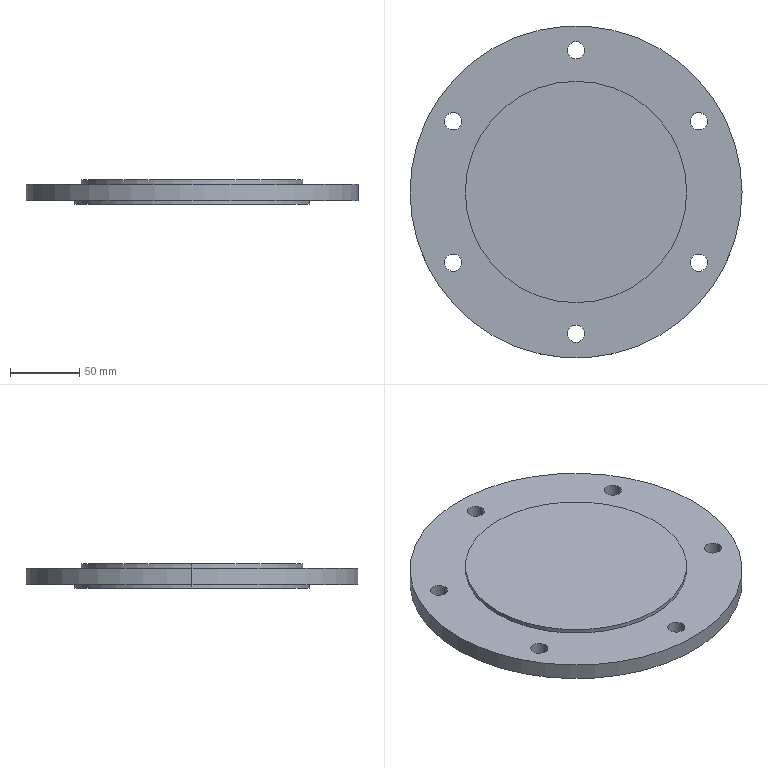Part | SolidWorks | features ICE 3, HoleWzd 2, Revolution 1 | 1 solid | 28 faces | box 240 x 240 x 17.5 mm | volume 563209 mm3 | cylinder 22 | plane 6 | commonest cylinder face diameters 12.5 x12 100 x2 130 x2 160 x2 170 x2 240 x2
STEP:
#1=CARTESIAN_POINT('',(586.231,234.744,-152.193));
#2=VERTEX_POINT('',#1);
#3=CARTESIAN_POINT('',(456.231,234.744,-152.193));
#4=VERTEX_POINT('',#3);
#5=CARTESIAN_POINT('',(521.231,234.744,-152.193));
#6=DIRECTION('',(0.,0.,-1.));
#7=DIRECTION('',(-1.,0.,0.));
#8=AXIS2_PLACEMENT_3D('',#5,#6,#7);
#9=CIRCLE('',#8,65.);
#10=EDGE_CURVE('',#2,#4,#9,.T.);
#11=ORIENTED_EDGE('',*,*,#10,.F.);
#12=CARTESIAN_POINT('',(586.231,234.744,-153.193));
#13=VERTEX_POINT('',#12);
#14=CARTESIAN_POINT('',(586.231,234.744,-153.193));
#15=DIRECTION('',(0.,0.,-1.));
#16=VECTOR('',#15,1000.);
#17=LINE('',#14,#16);
#18=EDGE_CURVE('',#2,#13,#17,.T.);
#19=ORIENTED_EDGE('',*,*,#18,.T.);
#20=CARTESIAN_POINT('',(456.231,234.744,-153.193));
#21=VERTEX_POINT('',#20);
#22=CARTESIAN_POINT('',(521.231,234.744,-153.193));
#23=DIRECTION('',(0.,0.,-1.));
#24=DIRECTION('',(-1.,0.,0.));
#25=AXIS2_PLACEMENT_3D('',#22,#23,#24);
#26=CIRCLE('',#25,65.);
#27=EDGE_CURVE('',#13,#21,#26,.T.);
#28=ORIENTED_EDGE('',*,*,#27,.T.);
#29=CARTESIAN_POINT('',(456.231,234.744,-153.193));
#30=DIRECTION('',(0.,0.,-1.));
#31=VECTOR('',#30,1000.);
#32=LINE('',#29,#31);
#33=EDGE_CURVE('',#4,#21,#32,.T.);
#34=ORIENTED_EDGE('',*,*,#33,.F.);
#35=EDGE_LOOP('',(#11,#19,#28,#34));
#36=FACE_OUTER_BOUND('',#35,.T.);
#37=CARTESIAN_POINT('',(521.231,234.744,-153.193));
#38=DIRECTION('',(0.,0.,-1.));
#39=DIRECTION('',(-1.,0.,0.));
#40=AXIS2_PLACEMENT_3D('',#37,#38,#39);
#41=CYLINDRICAL_SURFACE('',#40,65.);
#42=ADVANCED_FACE('',(#36),#41,.F.);
#43=CARTESIAN_POINT('',(527.481,337.244,-150.693));
#44=VERTEX_POINT('',#43);
#45=CARTESIAN_POINT('',(514.981,337.244,-150.693));
#46=VERTEX_POINT('',#45);
#47=CARTESIAN_POINT('',(521.231,337.244,-150.693));
#48=DIRECTION('',(0.,0.,-1.));
#49=DIRECTION('',(-1.,0.,0.));
#50=AXIS2_PLACEMENT_3D('',#47,#48,#49);
#51=CIRCLE('',#50,6.25);
#52=EDGE_CURVE('',#44,#46,#51,.T.);
#53=ORIENTED_EDGE('',*,*,#52,.T.);
#54=CARTESIAN_POINT('',(514.981,337.244,-138.693));
#55=VERTEX_POINT('',#54);
#56=CARTESIAN_POINT('',(514.981,337.244,-138.693));
#57=DIRECTION('',(0.,0.,1.));
#58=VECTOR('',#57,1000.);
#59=LINE('',#56,#58);
#60=EDGE_CURVE('',#46,#55,#59,.T.);
#61=ORIENTED_EDGE('',*,*,#60,.T.);
#62=CARTESIAN_POINT('',(527.481,337.244,-138.693));
#63=VERTEX_POINT('',#62);
#64=CARTESIAN_POINT('',(521.231,337.244,-138.693));
#65=DIRECTION('',(0.,0.,1.));
#66=DIRECTION('',(1.,0.,0.));
#67=AXIS2_PLACEMENT_3D('',#64,#65,#66);
#68=CIRCLE('',#67,6.25);
#69=EDGE_CURVE('',#55,#63,#68,.T.);
#70=ORIENTED_EDGE('',*,*,#69,.T.);
#71=CARTESIAN_POINT('',(527.481,337.244,-138.693));
#72=DIRECTION('',(0.,0.,1.));
#73=VECTOR('',#72,1000.);
#74=LINE('',#71,#73);
#75=EDGE_CURVE('',#44,#63,#74,.T.);
#76=ORIENTED_EDGE('',*,*,#75,.F.);
#77=EDGE_LOOP('',(#53,#61,#70,#76));
#78=FACE_OUTER_BOUND('',#77,.T.);
#79=CARTESIAN_POINT('',(521.231,337.244,-138.693));
#80=DIRECTION('',(0.,0.,1.));
#81=DIRECTION('',(1.,0.,0.));
#82=AXIS2_PLACEMENT_3D('',#79,#80,#81);
#83=CYLINDRICAL_SURFACE('',#82,6.25);
#84=ADVANCED_FACE('',(#78),#83,.F.);
#85=CARTESIAN_POINT('',(616.248,285.994,-150.693));
#86=VERTEX_POINT('',#85);
#87=CARTESIAN_POINT('',(603.748,285.994,-150.693));
#88=VERTEX_POINT('',#87);
#89=CARTESIAN_POINT('',(609.998,285.994,-150.693));
#90=DIRECTION('',(0.,0.,-1.));
#91=DIRECTION('',(-1.,0.,0.));
#92=AXIS2_PLACEMENT_3D('',#89,#90,#91);
#93=CIRCLE('',#92,6.25);
#94=EDGE_CURVE('',#86,#88,#93,.T.);
#95=ORIENTED_EDGE('',*,*,#94,.T.);
#96=CARTESIAN_POINT('',(603.748,285.994,-138.693));
#97=VERTEX_POINT('',#96);
#98=CARTESIAN_POINT('',(603.748,285.994,-138.693));
#99=DIRECTION('',(0.,0.,1.));
#100=VECTOR('',#99,1000.);
#101=LINE('',#98,#100);
#102=EDGE_CURVE('',#88,#97,#101,.T.);
#103=ORIENTED_EDGE('',*,*,#102,.T.);
#104=CARTESIAN_POINT('',(616.248,285.994,-138.693));
#105=VERTEX_POINT('',#104);
#106=CARTESIAN_POINT('',(609.998,285.994,-138.693));
#107=DIRECTION('',(0.,0.,1.));
#108=DIRECTION('',(1.,0.,0.));
#109=AXIS2_PLACEMENT_3D('',#106,#107,#108);
#110=CIRCLE('',#109,6.25);
#111=EDGE_CURVE('',#97,#105,#110,.T.);
#112=ORIENTED_EDGE('',*,*,#111,.T.);
#113=CARTESIAN_POINT('',(616.248,285.994,-138.693));
#114=DIRECTION('',(0.,0.,1.));
#115=VECTOR('',#114,1000.);
#116=LINE('',#113,#115);
#117=EDGE_CURVE('',#86,#105,#116,.T.);
#118=ORIENTED_EDGE('',*,*,#117,.F.);
#119=EDGE_LOOP('',(#95,#103,#112,#118));
#120=FACE_OUTER_BOUND('',#119,.T.);
#121=CARTESIAN_POINT('',(609.998,285.994,-138.693));
#122=DIRECTION('',(0.,0.,1.));
#123=DIRECTION('',(1.,0.,0.));
#124=AXIS2_PLACEMENT_3D('',#121,#122,#123);
#125=CYLINDRICAL_SURFACE('',#124,6.25);
#126=ADVANCED_FACE('',(#120),#125,.F.);
#127=CARTESIAN_POINT('',(438.713,285.994,-150.693));
#128=VERTEX_POINT('',#127);
#129=CARTESIAN_POINT('',(426.213,285.994,-150.693));
#130=VERTEX_POINT('',#129);
#131=CARTESIAN_POINT('',(432.463,285.994,-150.693));
#132=DIRECTION('',(0.,0.,-1.));
#133=DIRECTION('',(-1.,0.,0.));
#134=AXIS2_PLACEMENT_3D('',#131,#132,#133);
#135=CIRCLE('',#134,6.25);
#136=EDGE_CURVE('',#128,#130,#135,.T.);
#137=ORIENTED_EDGE('',*,*,#136,.T.);
#138=CARTESIAN_POINT('',(426.213,285.994,-138.693));
#139=VERTEX_POINT('',#138);
#140=CARTESIAN_POINT('',(426.213,285.994,-138.693));
#141=DIRECTION('',(0.,0.,1.));
#142=VECTOR('',#141,1000.);
#143=LINE('',#140,#142);
#144=EDGE_CURVE('',#130,#139,#143,.T.);
#145=ORIENTED_EDGE('',*,*,#144,.T.);
#146=CARTESIAN_POINT('',(438.713,285.994,-138.693));
#147=VERTEX_POINT('',#146);
#148=CARTESIAN_POINT('',(432.463,285.994,-138.693));
#149=DIRECTION('',(0.,0.,1.));
#150=DIRECTION('',(1.,0.,0.));
#151=AXIS2_PLACEMENT_3D('',#148,#149,#150);
#152=CIRCLE('',#151,6.25);
#153=EDGE_CURVE('',#139,#147,#152,.T.);
#154=ORIENTED_EDGE('',*,*,#153,.T.);
#155=CARTESIAN_POINT('',(438.713,285.994,-138.693));
#156=DIRECTION('',(0.,0.,1.));
#157=VECTOR('',#156,1000.);
#158=LINE('',#155,#157);
#159=EDGE_CURVE('',#128,#147,#158,.T.);
#160=ORIENTED_EDGE('',*,*,#159,.F.);
#161=EDGE_LOOP('',(#137,#145,#154,#160));
#162=FACE_OUTER_BOUND('',#161,.T.);
#163=CARTESIAN_POINT('',(432.463,285.994,-138.693));
#164=DIRECTION('',(0.,0.,1.));
#165=DIRECTION('',(1.,0.,0.));
#166=AXIS2_PLACEMENT_3D('',#163,#164,#165);
#167=CYLINDRICAL_SURFACE('',#166,6.25);
#168=ADVANCED_FACE('',(#162),#167,.F.);
#169=CARTESIAN_POINT('',(438.713,183.494,-150.693));
#170=VERTEX_POINT('',#169);
#171=CARTESIAN_POINT('',(426.213,183.494,-150.693));
#172=VERTEX_POINT('',#171);
#173=CARTESIAN_POINT('',(432.463,183.494,-150.693));
#174=DIRECTION('',(0.,0.,-1.));
#175=DIRECTION('',(-1.,0.,0.));
#176=AXIS2_PLACEMENT_3D('',#173,#174,#175);
#177=CIRCLE('',#176,6.25);
#178=EDGE_CURVE('',#170,#172,#177,.T.);
#179=ORIENTED_EDGE('',*,*,#178,.T.);
#180=CARTESIAN_POINT('',(426.213,183.494,-138.693));
#181=VERTEX_POINT('',#180);
#182=CARTESIAN_POINT('',(426.213,183.494,-138.693));
#183=DIRECTION('',(0.,0.,1.));
#184=VECTOR('',#183,1000.);
#185=LINE('',#182,#184);
#186=EDGE_CURVE('',#172,#181,#185,.T.);
#187=ORIENTED_EDGE('',*,*,#186,.T.);
#188=CARTESIAN_POINT('',(438.713,183.494,-138.693));
#189=VERTEX_POINT('',#188);
#190=CARTESIAN_POINT('',(432.463,183.494,-138.693));
#191=DIRECTION('',(0.,0.,1.));
#192=DIRECTION('',(1.,0.,0.));
#193=AXIS2_PLACEMENT_3D('',#190,#191,#192);
#194=CIRCLE('',#193,6.25);
#195=EDGE_CURVE('',#181,#189,#194,.T.);
#196=ORIENTED_EDGE('',*,*,#195,.T.);
#197=CARTESIAN_POINT('',(438.713,183.494,-138.693));
#198=DIRECTION('',(0.,0.,1.));
#199=VECTOR('',#198,1000.);
#200=LINE('',#197,#199);
#201=EDGE_CURVE('',#170,#189,#200,.T.);
#202=ORIENTED_EDGE('',*,*,#201,.F.);
#203=EDGE_LOOP('',(#179,#187,#196,#202));
#204=FACE_OUTER_BOUND('',#203,.T.);
#205=CARTESIAN_POINT('',(432.463,183.494,-138.693));
#206=DIRECTION('',(0.,0.,1.));
#207=DIRECTION('',(1.,0.,0.));
#208=AXIS2_PLACEMENT_3D('',#205,#206,#207);
#209=CYLINDRICAL_SURFACE('',#208,6.25);
#210=ADVANCED_FACE('',(#204),#209,.F.);
#211=CARTESIAN_POINT('',(527.481,132.244,-150.693));
#212=VERTEX_POINT('',#211);
#213=CARTESIAN_POINT('',(514.981,132.244,-150.693));
#214=VERTEX_POINT('',#213);
#215=CARTESIAN_POINT('',(521.231,132.244,-150.693));
#216=DIRECTION('',(0.,0.,-1.));
#217=DIRECTION('',(-1.,0.,0.));
#218=AXIS2_PLACEMENT_3D('',#215,#216,#217);
#219=CIRCLE('',#218,6.25);
#220=EDGE_CURVE('',#212,#214,#219,.T.);
#221=ORIENTED_EDGE('',*,*,#220,.T.);
#222=CARTESIAN_POINT('',(514.981,132.244,-138.693));
#223=VERTEX_POINT('',#222);
#224=CARTESIAN_POINT('',(514.981,132.244,-138.693));
#225=DIRECTION('',(0.,0.,1.));
#226=VECTOR('',#225,1000.);
#227=LINE('',#224,#226);
#228=EDGE_CURVE('',#214,#223,#227,.T.);
#229=ORIENTED_EDGE('',*,*,#228,.T.);
#230=CARTESIAN_POINT('',(527.481,132.244,-138.693));
#231=VERTEX_POINT('',#230);
#232=CARTESIAN_POINT('',(521.231,132.244,-138.693));
#233=DIRECTION('',(0.,0.,1.));
#234=DIRECTION('',(1.,0.,0.));
#235=AXIS2_PLACEMENT_3D('',#232,#233,#234);
#236=CIRCLE('',#235,6.25);
#237=EDGE_CURVE('',#223,#231,#236,.T.);
#238=ORIENTED_EDGE('',*,*,#237,.T.);
#239=CARTESIAN_POINT('',(527.481,132.244,-138.693));
#240=DIRECTION('',(0.,0.,1.));
#241=VECTOR('',#240,1000.);
#242=LINE('',#239,#241);
#243=EDGE_CURVE('',#212,#231,#242,.T.);
#244=ORIENTED_EDGE('',*,*,#243,.F.);
#245=EDGE_LOOP('',(#221,#229,#238,#244));
#246=FACE_OUTER_BOUND('',#245,.T.);
#247=CARTESIAN_POINT('',(521.231,132.244,-138.693));
#248=DIRECTION('',(0.,0.,1.));
#249=DIRECTION('',(1.,0.,0.));
#250=AXIS2_PLACEMENT_3D('',#247,#248,#249);
#251=CYLINDRICAL_SURFACE('',#250,6.25);
#252=ADVANCED_FACE('',(#246),#251,.F.);
#253=CARTESIAN_POINT('',(616.248,183.494,-150.693));
#254=VERTEX_POINT('',#253);
#255=CARTESIAN_POINT('',(603.748,183.494,-150.693));
#256=VERTEX_POINT('',#255);
#257=CARTESIAN_POINT('',(609.998,183.494,-150.693));
#258=DIRECTION('',(0.,0.,-1.));
#259=DIRECTION('',(-1.,0.,0.));
#260=AXIS2_PLACEMENT_3D('',#257,#258,#259);
#261=CIRCLE('',#260,6.25);
#262=EDGE_CURVE('',#254,#256,#261,.T.);
#263=ORIENTED_EDGE('',*,*,#262,.T.);
#264=CARTESIAN_POINT('',(603.748,183.494,-138.693));
#265=VERTEX_POINT('',#264);
#266=CARTESIAN_POINT('',(603.748,183.494,-138.693));
#267=DIRECTION('',(0.,0.,1.));
#268=VECTOR('',#267,1000.);
#269=LINE('',#266,#268);
#270=EDGE_CURVE('',#256,#265,#269,.T.);
#271=ORIENTED_EDGE('',*,*,#270,.T.);
#272=CARTESIAN_POINT('',(616.248,183.494,-138.693));
#273=VERTEX_POINT('',#272);
#274=CARTESIAN_POINT('',(609.998,183.494,-138.693));
#275=DIRECTION('',(0.,0.,1.));
#276=DIRECTION('',(1.,0.,0.));
#277=AXIS2_PLACEMENT_3D('',#274,#275,#276);
#278=CIRCLE('',#277,6.25);
#279=EDGE_CURVE('',#265,#273,#278,.T.);
#280=ORIENTED_EDGE('',*,*,#279,.T.);
#281=CARTESIAN_POINT('',(616.248,183.494,-138.693));
#282=DIRECTION('',(0.,0.,1.));
#283=VECTOR('',#282,1000.);
#284=LINE('',#281,#283);
#285=EDGE_CURVE('',#254,#273,#284,.T.);
#286=ORIENTED_EDGE('',*,*,#285,.F.);
#287=EDGE_LOOP('',(#263,#271,#280,#286));
#288=FACE_OUTER_BOUND('',#287,.T.);
#289=CARTESIAN_POINT('',(609.998,183.494,-138.693));
#290=DIRECTION('',(0.,0.,1.));
#291=DIRECTION('',(1.,0.,0.));
#292=AXIS2_PLACEMENT_3D('',#289,#290,#291);
#293=CYLINDRICAL_SURFACE('',#292,6.25);
#294=ADVANCED_FACE('',(#288),#293,.F.);
#295=CARTESIAN_POINT('',(601.231,234.744,-135.693));
#296=VERTEX_POINT('',#295);
#297=CARTESIAN_POINT('',(441.231,234.744,-135.693));
#298=VERTEX_POINT('',#297);
#299=CARTESIAN_POINT('',(521.231,234.744,-135.693));
#300=DIRECTION('',(0.,0.,1.));
#301=DIRECTION('',(1.,0.,0.));
#302=AXIS2_PLACEMENT_3D('',#299,#300,#301);
#303=CIRCLE('',#302,80.);
#304=EDGE_CURVE('',#296,#298,#303,.T.);
#305=ORIENTED_EDGE('',*,*,#304,.F.);
#306=CARTESIAN_POINT('',(601.231,234.744,-138.693));
#307=VERTEX_POINT('',#306);
#308=CARTESIAN_POINT('',(601.231,234.744,-135.693));
#309=DIRECTION('',(0.,0.,-1.));
#310=VECTOR('',#309,1000.);
#311=LINE('',#308,#310);
#312=EDGE_CURVE('',#296,#307,#311,.T.);
#313=ORIENTED_EDGE('',*,*,#312,.T.);
#314=CARTESIAN_POINT('',(441.231,234.744,-138.693));
#315=VERTEX_POINT('',#314);
#316=CARTESIAN_POINT('',(521.231,234.744,-138.693));
#317=DIRECTION('',(0.,0.,1.));
#318=DIRECTION('',(1.,0.,0.));
#319=AXIS2_PLACEMENT_3D('',#316,#317,#318);
#320=CIRCLE('',#319,80.);
#321=EDGE_CURVE('',#307,#315,#320,.T.);
#322=ORIENTED_EDGE('',*,*,#321,.T.);
#323=CARTESIAN_POINT('',(441.231,234.744,-135.693));
#324=DIRECTION('',(0.,0.,-1.));
#325=VECTOR('',#324,1000.);
#326=LINE('',#323,#325);
#327=EDGE_CURVE('',#298,#315,#326,.T.);
#328=ORIENTED_EDGE('',*,*,#327,.F.);
#329=EDGE_LOOP('',(#305,#313,#322,#328));
#330=FACE_OUTER_BOUND('',#329,.T.);
#331=CARTESIAN_POINT('',(521.231,234.744,-135.693));
#332=DIRECTION('',(0.,0.,-1.));
#333=DIRECTION('',(-1.,0.,0.));
#334=AXIS2_PLACEMENT_3D('',#331,#332,#333);
#335=CYLINDRICAL_SURFACE('',#334,80.);
#336=ADVANCED_FACE('',(#330),#335,.T.);
#337=CARTESIAN_POINT('',(436.231,234.744,-153.193));
#338=VERTEX_POINT('',#337);
#339=CARTESIAN_POINT('',(606.231,234.744,-153.193));
#340=VERTEX_POINT('',#339);
#341=CARTESIAN_POINT('',(521.231,234.744,-153.193));
#342=DIRECTION('',(0.,0.,-1.));
#343=DIRECTION('',(-1.,0.,0.));
#344=AXIS2_PLACEMENT_3D('',#341,#342,#343);
#345=CIRCLE('',#344,85.);
#346=EDGE_CURVE('',#338,#340,#345,.T.);
#347=ORIENTED_EDGE('',*,*,#346,.F.);
#348=CARTESIAN_POINT('',(436.231,234.744,-150.693));
#349=VERTEX_POINT('',#348);
#350=CARTESIAN_POINT('',(436.231,234.744,-153.193));
#351=DIRECTION('',(0.,0.,1.));
#352=VECTOR('',#351,1000.);
#353=LINE('',#350,#352);
#354=EDGE_CURVE('',#338,#349,#353,.T.);
#355=ORIENTED_EDGE('',*,*,#354,.T.);
#356=CARTESIAN_POINT('',(606.231,234.744,-150.693));
#357=VERTEX_POINT('',#356);
#358=CARTESIAN_POINT('',(521.231,234.744,-150.693));
#359=DIRECTION('',(0.,0.,-1.));
#360=DIRECTION('',(-1.,0.,0.));
#361=AXIS2_PLACEMENT_3D('',#358,#359,#360);
#362=CIRCLE('',#361,85.);
#363=EDGE_CURVE('',#349,#357,#362,.T.);
#364=ORIENTED_EDGE('',*,*,#363,.T.);
#365=CARTESIAN_POINT('',(606.231,234.744,-153.193));
#366=DIRECTION('',(0.,0.,1.));
#367=VECTOR('',#366,1000.);
#368=LINE('',#365,#367);
#369=EDGE_CURVE('',#340,#357,#368,.T.);
#370=ORIENTED_EDGE('',*,*,#369,.F.);
#371=EDGE_LOOP('',(#347,#355,#364,#370));
#372=FACE_OUTER_BOUND('',#371,.T.);
#373=CARTESIAN_POINT('',(521.231,234.744,-153.193));
#374=DIRECTION('',(0.,0.,1.));
#375=DIRECTION('',(1.,0.,0.));
#376=AXIS2_PLACEMENT_3D('',#373,#374,#375);
#377=CYLINDRICAL_SURFACE('',#376,85.);
#378=ADVANCED_FACE('',(#372),#377,.T.);
#379=CARTESIAN_POINT('',(641.231,234.744,-150.693));
#380=VERTEX_POINT('',#379);
#381=CARTESIAN_POINT('',(401.231,234.744,-150.693));
#382=VERTEX_POINT('',#381);
#383=CARTESIAN_POINT('',(521.231,234.744,-150.693));
#384=DIRECTION('',(0.,0.,1.));
#385=DIRECTION('',(1.,0.,0.));
#386=AXIS2_PLACEMENT_3D('',#383,#384,#385);
#387=CIRCLE('',#386,120.);
#388=EDGE_CURVE('',#380,#382,#387,.T.);
#389=ORIENTED_EDGE('',*,*,#388,.T.);
#390=CARTESIAN_POINT('',(401.231,234.744,-138.693));
#391=VERTEX_POINT('',#390);
#392=CARTESIAN_POINT('',(401.231,234.744,-150.693));
#393=DIRECTION('',(0.,0.,1.));
#394=VECTOR('',#393,1000.);
#395=LINE('',#392,#394);
#396=EDGE_CURVE('',#382,#391,#395,.T.);
#397=ORIENTED_EDGE('',*,*,#396,.T.);
#398=CARTESIAN_POINT('',(641.231,234.744,-138.693));
#399=VERTEX_POINT('',#398);
#400=CARTESIAN_POINT('',(521.231,234.744,-138.693));
#401=DIRECTION('',(0.,0.,1.));
#402=DIRECTION('',(1.,0.,0.));
#403=AXIS2_PLACEMENT_3D('',#400,#401,#402);
#404=CIRCLE('',#403,120.);
#405=EDGE_CURVE('',#399,#391,#404,.T.);
#406=ORIENTED_EDGE('',*,*,#405,.F.);
#407=CARTESIAN_POINT('',(641.231,234.744,-150.693));
#408=DIRECTION('',(0.,0.,1.));
#409=VECTOR('',#408,1000.);
#410=LINE('',#407,#409);
#411=EDGE_CURVE('',#380,#399,#410,.T.);
#412=ORIENTED_EDGE('',*,*,#411,.F.);
#413=EDGE_LOOP('',(#389,#397,#406,#412));
#414=FACE_OUTER_BOUND('',#413,.T.);
#415=CARTESIAN_POINT('',(521.231,234.744,-150.693));
#416=DIRECTION('',(0.,0.,1.));
#417=DIRECTION('',(1.,0.,0.));
#418=AXIS2_PLACEMENT_3D('',#415,#416,#417);
#419=CYLINDRICAL_SURFACE('',#418,120.);
#420=ADVANCED_FACE('',(#414),#419,.T.);
#421=CARTESIAN_POINT('',(571.231,234.744,-142.693));
#422=VERTEX_POINT('',#421);
#423=CARTESIAN_POINT('',(471.231,234.744,-142.693));
#424=VERTEX_POINT('',#423);
#425=CARTESIAN_POINT('',(521.231,234.744,-142.693));
#426=DIRECTION('',(0.,0.,-1.));
#427=DIRECTION('',(1.,0.,0.));
#428=AXIS2_PLACEMENT_3D('',#425,#426,#427);
#429=CIRCLE('',#428,50.);
#430=EDGE_CURVE('',#422,#424,#429,.T.);
#431=ORIENTED_EDGE('',*,*,#430,.F.);
#432=CARTESIAN_POINT('',(571.231,234.744,-152.193));
#433=VERTEX_POINT('',#432);
#434=CARTESIAN_POINT('',(571.231,234.744,-153.193));
#435=DIRECTION('',(0.,0.,-1.));
#436=VECTOR('',#435,1000.);
#437=LINE('',#434,#436);
#438=EDGE_CURVE('',#422,#433,#437,.T.);
#439=ORIENTED_EDGE('',*,*,#438,.T.);
#440=CARTESIAN_POINT('',(471.231,234.744,-152.193));
#441=VERTEX_POINT('',#440);
#442=CARTESIAN_POINT('',(521.231,234.744,-152.193));
#443=DIRECTION('',(0.,0.,-1.));
#444=DIRECTION('',(-1.,0.,0.));
#445=AXIS2_PLACEMENT_3D('',#442,#443,#444);
#446=CIRCLE('',#445,50.);
#447=EDGE_CURVE('',#433,#441,#446,.T.);
#448=ORIENTED_EDGE('',*,*,#447,.T.);
#449=CARTESIAN_POINT('',(471.231,234.744,-153.193));
#450=DIRECTION('',(0.,0.,-1.));
#451=VECTOR('',#450,1000.);
#452=LINE('',#449,#451);
#453=EDGE_CURVE('',#424,#441,#452,.T.);
#454=ORIENTED_EDGE('',*,*,#453,.F.);
#455=EDGE_LOOP('',(#431,#439,#448,#454));
#456=FACE_OUTER_BOUND('',#455,.T.);
#457=CARTESIAN_POINT('',(521.231,234.744,-153.193));
#458=DIRECTION('',(0.,0.,-1.));
#459=DIRECTION('',(-1.,0.,0.));
#460=AXIS2_PLACEMENT_3D('',#457,#458,#459);
#461=CYLINDRICAL_SURFACE('',#460,50.);
#462=ADVANCED_FACE('',(#456),#461,.F.);
#463=ORIENTED_EDGE('',*,*,#438,.F.);
#464=CARTESIAN_POINT('',(521.231,234.744,-142.693));
#465=DIRECTION('',(0.,0.,-1.));
#466=DIRECTION('',(1.,0.,0.));
#467=AXIS2_PLACEMENT_3D('',#464,#465,#466);
#468=CIRCLE('',#467,50.);
#469=EDGE_CURVE('',#424,#422,#468,.T.);
#470=ORIENTED_EDGE('',*,*,#469,.F.);
#471=ORIENTED_EDGE('',*,*,#453,.T.);
#472=CARTESIAN_POINT('',(521.231,234.744,-152.193));
#473=DIRECTION('',(0.,0.,-1.));
#474=DIRECTION('',(-1.,0.,0.));
#475=AXIS2_PLACEMENT_3D('',#472,#473,#474);
#476=CIRCLE('',#475,50.);
#477=EDGE_CURVE('',#441,#433,#476,.T.);
#478=ORIENTED_EDGE('',*,*,#477,.T.);
#479=EDGE_LOOP('',(#463,#470,#471,#478));
#480=FACE_OUTER_BOUND('',#479,.T.);
#481=CARTESIAN_POINT('',(521.231,234.744,-153.193));
#482=DIRECTION('',(0.,0.,-1.));
#483=DIRECTION('',(-1.,0.,0.));
#484=AXIS2_PLACEMENT_3D('',#481,#482,#483);
#485=CYLINDRICAL_SURFACE('',#484,50.);
#486=ADVANCED_FACE('',(#480),#485,.F.);
#487=ORIENTED_EDGE('',*,*,#396,.F.);
#488=CARTESIAN_POINT('',(521.231,234.744,-150.693));
#489=DIRECTION('',(0.,0.,1.));
#490=DIRECTION('',(1.,0.,0.));
#491=AXIS2_PLACEMENT_3D('',#488,#489,#490);
#492=CIRCLE('',#491,120.);
#493=EDGE_CURVE('',#382,#380,#492,.T.);
#494=ORIENTED_EDGE('',*,*,#493,.T.);
#495=ORIENTED_EDGE('',*,*,#411,.T.);
#496=CARTESIAN_POINT('',(521.231,234.744,-138.693));
#497=DIRECTION('',(0.,0.,1.));
#498=DIRECTION('',(1.,0.,0.));
#499=AXIS2_PLACEMENT_3D('',#496,#497,#498);
#500=CIRCLE('',#499,120.);
#501=EDGE_CURVE('',#391,#399,#500,.T.);
#502=ORIENTED_EDGE('',*,*,#501,.F.);
#503=EDGE_LOOP('',(#487,#494,#495,#502));
#504=FACE_OUTER_BOUND('',#503,.T.);
#505=CARTESIAN_POINT('',(521.231,234.744,-150.693));
#506=DIRECTION('',(0.,0.,1.));
#507=DIRECTION('',(1.,0.,0.));
#508=AXIS2_PLACEMENT_3D('',#505,#506,#507);
#509=CYLINDRICAL_SURFACE('',#508,120.);
#510=ADVANCED_FACE('',(#504),#509,.T.);
#511=ORIENTED_EDGE('',*,*,#52,.F.);
#512=CARTESIAN_POINT('',(521.231,337.244,-150.693));
#513=DIRECTION('',(0.,0.,-1.));
#514=DIRECTION('',(-1.,0.,0.));
#515=AXIS2_PLACEMENT_3D('',#512,#513,#514);
#516=CIRCLE('',#515,6.25);
#517=EDGE_CURVE('',#46,#44,#516,.T.);
#518=ORIENTED_EDGE('',*,*,#517,.F.);
#519=EDGE_LOOP('',(#511,#518));
#520=FACE_BOUND('',#519,.T.);
#521=ORIENTED_EDGE('',*,*,#94,.F.);
#522=CARTESIAN_POINT('',(609.998,285.994,-150.693));
#523=DIRECTION('',(0.,0.,-1.));
#524=DIRECTION('',(-1.,0.,0.));
#525=AXIS2_PLACEMENT_3D('',#522,#523,#524);
#526=CIRCLE('',#525,6.25);
#527=EDGE_CURVE('',#88,#86,#526,.T.);
#528=ORIENTED_EDGE('',*,*,#527,.F.);
#529=EDGE_LOOP('',(#521,#528));
#530=FACE_BOUND('',#529,.T.);
#531=ORIENTED_EDGE('',*,*,#136,.F.);
#532=CARTESIAN_POINT('',(432.463,285.994,-150.693));
#533=DIRECTION('',(0.,0.,-1.));
#534=DIRECTION('',(-1.,0.,0.));
#535=AXIS2_PLACEMENT_3D('',#532,#533,#534);
#536=CIRCLE('',#535,6.25);
#537=EDGE_CURVE('',#130,#128,#536,.T.);
#538=ORIENTED_EDGE('',*,*,#537,.F.);
#539=EDGE_LOOP('',(#531,#538));
#540=FACE_BOUND('',#539,.T.);
#541=ORIENTED_EDGE('',*,*,#178,.F.);
#542=CARTESIAN_POINT('',(432.463,183.494,-150.693));
#543=DIRECTION('',(0.,0.,-1.));
#544=DIRECTION('',(-1.,0.,0.));
#545=AXIS2_PLACEMENT_3D('',#542,#543,#544);
#546=CIRCLE('',#545,6.25);
#547=EDGE_CURVE('',#172,#170,#546,.T.);
#548=ORIENTED_EDGE('',*,*,#547,.F.);
#549=EDGE_LOOP('',(#541,#548));
#550=FACE_BOUND('',#549,.T.);
#551=ORIENTED_EDGE('',*,*,#220,.F.);
#552=CARTESIAN_POINT('',(521.231,132.244,-150.693));
#553=DIRECTION('',(0.,0.,-1.));
#554=DIRECTION('',(-1.,0.,0.));
#555=AXIS2_PLACEMENT_3D('',#552,#553,#554);
#556=CIRCLE('',#555,6.25);
#557=EDGE_CURVE('',#214,#212,#556,.T.);
#558=ORIENTED_EDGE('',*,*,#557,.F.);
#559=EDGE_LOOP('',(#551,#558));
#560=FACE_BOUND('',#559,.T.);
#561=ORIENTED_EDGE('',*,*,#262,.F.);
#562=CARTESIAN_POINT('',(609.998,183.494,-150.693));
#563=DIRECTION('',(0.,0.,-1.));
#564=DIRECTION('',(-1.,0.,0.));
#565=AXIS2_PLACEMENT_3D('',#562,#563,#564);
#566=CIRCLE('',#565,6.25);
#567=EDGE_CURVE('',#256,#254,#566,.T.);
#568=ORIENTED_EDGE('',*,*,#567,.F.);
#569=EDGE_LOOP('',(#561,#568));
#570=FACE_BOUND('',#569,.T.);
#571=CARTESIAN_POINT('',(521.231,234.744,-150.693));
#572=DIRECTION('',(0.,0.,-1.));
#573=DIRECTION('',(-1.,0.,0.));
#574=AXIS2_PLACEMENT_3D('',#571,#572,#573);
#575=CIRCLE('',#574,85.);
#576=EDGE_CURVE('',#357,#349,#575,.T.);
#577=ORIENTED_EDGE('',*,*,#576,.F.);
#578=ORIENTED_EDGE('',*,*,#363,.F.);
#579=EDGE_LOOP('',(#577,#578));
#580=FACE_BOUND('',#579,.T.);
#581=ORIENTED_EDGE('',*,*,#388,.F.);
#582=ORIENTED_EDGE('',*,*,#493,.F.);
#583=EDGE_LOOP('',(#581,#582));
#584=FACE_OUTER_BOUND('',#583,.T.);
#585=CARTESIAN_POINT('',(641.231,234.744,-150.693));
#586=DIRECTION('',(0.,0.,-1.));
#587=DIRECTION('',(-1.,0.,0.));
#588=AXIS2_PLACEMENT_3D('',#585,#586,#587);
#589=PLANE('',#588);
#590=ADVANCED_FACE('',(#520,#530,#540,#550,#560,#570,#580,#584),#589,.T.);
#591=CARTESIAN_POINT('',(521.231,337.244,-138.693));
#592=DIRECTION('',(0.,0.,1.));
#593=DIRECTION('',(1.,0.,0.));
#594=AXIS2_PLACEMENT_3D('',#591,#592,#593);
#595=CIRCLE('',#594,6.25);
#596=EDGE_CURVE('',#63,#55,#595,.T.);
#597=ORIENTED_EDGE('',*,*,#596,.F.);
#598=ORIENTED_EDGE('',*,*,#69,.F.);
#599=EDGE_LOOP('',(#597,#598));
#600=FACE_BOUND('',#599,.T.);
#601=CARTESIAN_POINT('',(609.998,285.994,-138.693));
#602=DIRECTION('',(0.,0.,1.));
#603=DIRECTION('',(1.,0.,0.));
#604=AXIS2_PLACEMENT_3D('',#601,#602,#603);
#605=CIRCLE('',#604,6.25);
#606=EDGE_CURVE('',#105,#97,#605,.T.);
#607=ORIENTED_EDGE('',*,*,#606,.F.);
#608=ORIENTED_EDGE('',*,*,#111,.F.);
#609=EDGE_LOOP('',(#607,#608));
#610=FACE_BOUND('',#609,.T.);
#611=CARTESIAN_POINT('',(432.463,285.994,-138.693));
#612=DIRECTION('',(0.,0.,1.));
#613=DIRECTION('',(1.,0.,0.));
#614=AXIS2_PLACEMENT_3D('',#611,#612,#613);
#615=CIRCLE('',#614,6.25);
#616=EDGE_CURVE('',#147,#139,#615,.T.);
#617=ORIENTED_EDGE('',*,*,#616,.F.);
#618=ORIENTED_EDGE('',*,*,#153,.F.);
#619=EDGE_LOOP('',(#617,#618));
#620=FACE_BOUND('',#619,.T.);
#621=CARTESIAN_POINT('',(432.463,183.494,-138.693));
#622=DIRECTION('',(0.,0.,1.));
#623=DIRECTION('',(1.,0.,0.));
#624=AXIS2_PLACEMENT_3D('',#621,#622,#623);
#625=CIRCLE('',#624,6.25);
#626=EDGE_CURVE('',#189,#181,#625,.T.);
#627=ORIENTED_EDGE('',*,*,#626,.F.);
#628=ORIENTED_EDGE('',*,*,#195,.F.);
#629=EDGE_LOOP('',(#627,#628));
#630=FACE_BOUND('',#629,.T.);
#631=CARTESIAN_POINT('',(521.231,132.244,-138.693));
#632=DIRECTION('',(0.,0.,1.));
#633=DIRECTION('',(1.,0.,0.));
#634=AXIS2_PLACEMENT_3D('',#631,#632,#633);
#635=CIRCLE('',#634,6.25);
#636=EDGE_CURVE('',#231,#223,#635,.T.);
#637=ORIENTED_EDGE('',*,*,#636,.F.);
#638=ORIENTED_EDGE('',*,*,#237,.F.);
#639=EDGE_LOOP('',(#637,#638));
#640=FACE_BOUND('',#639,.T.);
#641=CARTESIAN_POINT('',(609.998,183.494,-138.693));
#642=DIRECTION('',(0.,0.,1.));
#643=DIRECTION('',(1.,0.,0.));
#644=AXIS2_PLACEMENT_3D('',#641,#642,#643);
#645=CIRCLE('',#644,6.25);
#646=EDGE_CURVE('',#273,#265,#645,.T.);
#647=ORIENTED_EDGE('',*,*,#646,.F.);
#648=ORIENTED_EDGE('',*,*,#279,.F.);
#649=EDGE_LOOP('',(#647,#648));
#650=FACE_BOUND('',#649,.T.);
#651=CARTESIAN_POINT('',(521.231,234.744,-138.693));
#652=DIRECTION('',(0.,0.,1.));
#653=DIRECTION('',(1.,0.,0.));
#654=AXIS2_PLACEMENT_3D('',#651,#652,#653);
#655=CIRCLE('',#654,80.);
#656=EDGE_CURVE('',#315,#307,#655,.T.);
#657=ORIENTED_EDGE('',*,*,#656,.F.);
#658=ORIENTED_EDGE('',*,*,#321,.F.);
#659=EDGE_LOOP('',(#657,#658));
#660=FACE_BOUND('',#659,.T.);
#661=ORIENTED_EDGE('',*,*,#405,.T.);
#662=ORIENTED_EDGE('',*,*,#501,.T.);
#663=EDGE_LOOP('',(#661,#662));
#664=FACE_OUTER_BOUND('',#663,.T.);
#665=CARTESIAN_POINT('',(521.231,234.744,-138.693));
#666=DIRECTION('',(0.,0.,1.));
#667=DIRECTION('',(1.,0.,0.));
#668=AXIS2_PLACEMENT_3D('',#665,#666,#667);
#669=PLANE('',#668);
#670=ADVANCED_FACE('',(#600,#610,#620,#630,#640,#650,#660,#664),#669,.T.);
#671=ORIENTED_EDGE('',*,*,#354,.F.);
#672=CARTESIAN_POINT('',(521.231,234.744,-153.193));
#673=DIRECTION('',(0.,0.,-1.));
#674=DIRECTION('',(-1.,0.,0.));
#675=AXIS2_PLACEMENT_3D('',#672,#673,#674);
#676=CIRCLE('',#675,85.);
#677=EDGE_CURVE('',#340,#338,#676,.T.);
#678=ORIENTED_EDGE('',*,*,#677,.F.);
#679=ORIENTED_EDGE('',*,*,#369,.T.);
#680=ORIENTED_EDGE('',*,*,#576,.T.);
#681=EDGE_LOOP('',(#671,#678,#679,#680));
#682=FACE_OUTER_BOUND('',#681,.T.);
#683=CARTESIAN_POINT('',(521.231,234.744,-153.193));
#684=DIRECTION('',(0.,0.,1.));
#685=DIRECTION('',(1.,0.,0.));
#686=AXIS2_PLACEMENT_3D('',#683,#684,#685);
#687=CYLINDRICAL_SURFACE('',#686,85.);
#688=ADVANCED_FACE('',(#682),#687,.T.);
#689=CARTESIAN_POINT('',(521.231,234.744,-153.193));
#690=DIRECTION('',(0.,0.,-1.));
#691=DIRECTION('',(-1.,0.,0.));
#692=AXIS2_PLACEMENT_3D('',#689,#690,#691);
#693=CIRCLE('',#692,65.);
#694=EDGE_CURVE('',#21,#13,#693,.T.);
#695=ORIENTED_EDGE('',*,*,#694,.F.);
#696=ORIENTED_EDGE('',*,*,#27,.F.);
#697=EDGE_LOOP('',(#695,#696));
#698=FACE_BOUND('',#697,.T.);
#699=ORIENTED_EDGE('',*,*,#677,.T.);
#700=ORIENTED_EDGE('',*,*,#346,.T.);
#701=EDGE_LOOP('',(#699,#700));
#702=FACE_OUTER_BOUND('',#701,.T.);
#703=CARTESIAN_POINT('',(521.231,234.744,-153.193));
#704=DIRECTION('',(0.,0.,-1.));
#705=DIRECTION('',(-1.,0.,0.));
#706=AXIS2_PLACEMENT_3D('',#703,#704,#705);
#707=PLANE('',#706);
#708=ADVANCED_FACE('',(#698,#702),#707,.T.);
#709=ORIENTED_EDGE('',*,*,#312,.F.);
#710=CARTESIAN_POINT('',(521.231,234.744,-135.693));
#711=DIRECTION('',(0.,0.,1.));
#712=DIRECTION('',(1.,0.,0.));
#713=AXIS2_PLACEMENT_3D('',#710,#711,#712);
#714=CIRCLE('',#713,80.);
#715=EDGE_CURVE('',#298,#296,#714,.T.);
#716=ORIENTED_EDGE('',*,*,#715,.F.);
#717=ORIENTED_EDGE('',*,*,#327,.T.);
#718=ORIENTED_EDGE('',*,*,#656,.T.);
#719=EDGE_LOOP('',(#709,#716,#717,#718));
#720=FACE_OUTER_BOUND('',#719,.T.);
#721=CARTESIAN_POINT('',(521.231,234.744,-135.693));
#722=DIRECTION('',(0.,0.,-1.));
#723=DIRECTION('',(-1.,0.,0.));
#724=AXIS2_PLACEMENT_3D('',#721,#722,#723);
#725=CYLINDRICAL_SURFACE('',#724,80.);
#726=ADVANCED_FACE('',(#720),#725,.T.);
#727=ORIENTED_EDGE('',*,*,#715,.T.);
#728=ORIENTED_EDGE('',*,*,#304,.T.);
#729=EDGE_LOOP('',(#727,#728));
#730=FACE_OUTER_BOUND('',#729,.T.);
#731=CARTESIAN_POINT('',(521.231,234.744,-135.693));
#732=DIRECTION('',(0.,0.,1.));
#733=DIRECTION('',(1.,0.,0.));
#734=AXIS2_PLACEMENT_3D('',#731,#732,#733);
#735=PLANE('',#734);
#736=ADVANCED_FACE('',(#730),#735,.T.);
#737=ORIENTED_EDGE('',*,*,#270,.F.);
#738=ORIENTED_EDGE('',*,*,#567,.T.);
#739=ORIENTED_EDGE('',*,*,#285,.T.);
#740=ORIENTED_EDGE('',*,*,#646,.T.);
#741=EDGE_LOOP('',(#737,#738,#739,#740));
#742=FACE_OUTER_BOUND('',#741,.T.);
#743=CARTESIAN_POINT('',(609.998,183.494,-138.693));
#744=DIRECTION('',(0.,0.,1.));
#745=DIRECTION('',(1.,0.,0.));
#746=AXIS2_PLACEMENT_3D('',#743,#744,#745);
#747=CYLINDRICAL_SURFACE('',#746,6.25);
#748=ADVANCED_FACE('',(#742),#747,.F.);
#749=ORIENTED_EDGE('',*,*,#228,.F.);
#750=ORIENTED_EDGE('',*,*,#557,.T.);
#751=ORIENTED_EDGE('',*,*,#243,.T.);
#752=ORIENTED_EDGE('',*,*,#636,.T.);
#753=EDGE_LOOP('',(#749,#750,#751,#752));
#754=FACE_OUTER_BOUND('',#753,.T.);
#755=CARTESIAN_POINT('',(521.231,132.244,-138.693));
#756=DIRECTION('',(0.,0.,1.));
#757=DIRECTION('',(1.,0.,0.));
#758=AXIS2_PLACEMENT_3D('',#755,#756,#757);
#759=CYLINDRICAL_SURFACE('',#758,6.25);
#760=ADVANCED_FACE('',(#754),#759,.F.);
#761=ORIENTED_EDGE('',*,*,#186,.F.);
#762=ORIENTED_EDGE('',*,*,#547,.T.);
#763=ORIENTED_EDGE('',*,*,#201,.T.);
#764=ORIENTED_EDGE('',*,*,#626,.T.);
#765=EDGE_LOOP('',(#761,#762,#763,#764));
#766=FACE_OUTER_BOUND('',#765,.T.);
#767=CARTESIAN_POINT('',(432.463,183.494,-138.693));
#768=DIRECTION('',(0.,0.,1.));
#769=DIRECTION('',(1.,0.,0.));
#770=AXIS2_PLACEMENT_3D('',#767,#768,#769);
#771=CYLINDRICAL_SURFACE('',#770,6.25);
#772=ADVANCED_FACE('',(#766),#771,.F.);
#773=ORIENTED_EDGE('',*,*,#144,.F.);
#774=ORIENTED_EDGE('',*,*,#537,.T.);
#775=ORIENTED_EDGE('',*,*,#159,.T.);
#776=ORIENTED_EDGE('',*,*,#616,.T.);
#777=EDGE_LOOP('',(#773,#774,#775,#776));
#778=FACE_OUTER_BOUND('',#777,.T.);
#779=CARTESIAN_POINT('',(432.463,285.994,-138.693));
#780=DIRECTION('',(0.,0.,1.));
#781=DIRECTION('',(1.,0.,0.));
#782=AXIS2_PLACEMENT_3D('',#779,#780,#781);
#783=CYLINDRICAL_SURFACE('',#782,6.25);
#784=ADVANCED_FACE('',(#778),#783,.F.);
#785=ORIENTED_EDGE('',*,*,#102,.F.);
#786=ORIENTED_EDGE('',*,*,#527,.T.);
#787=ORIENTED_EDGE('',*,*,#117,.T.);
#788=ORIENTED_EDGE('',*,*,#606,.T.);
#789=EDGE_LOOP('',(#785,#786,#787,#788));
#790=FACE_OUTER_BOUND('',#789,.T.);
#791=CARTESIAN_POINT('',(609.998,285.994,-138.693));
#792=DIRECTION('',(0.,0.,1.));
#793=DIRECTION('',(1.,0.,0.));
#794=AXIS2_PLACEMENT_3D('',#791,#792,#793);
#795=CYLINDRICAL_SURFACE('',#794,6.25);
#796=ADVANCED_FACE('',(#790),#795,.F.);
#797=ORIENTED_EDGE('',*,*,#60,.F.);
#798=ORIENTED_EDGE('',*,*,#517,.T.);
#799=ORIENTED_EDGE('',*,*,#75,.T.);
#800=ORIENTED_EDGE('',*,*,#596,.T.);
#801=EDGE_LOOP('',(#797,#798,#799,#800));
#802=FACE_OUTER_BOUND('',#801,.T.);
#803=CARTESIAN_POINT('',(521.231,337.244,-138.693));
#804=DIRECTION('',(0.,0.,1.));
#805=DIRECTION('',(1.,0.,0.));
#806=AXIS2_PLACEMENT_3D('',#803,#804,#805);
#807=CYLINDRICAL_SURFACE('',#806,6.25);
#808=ADVANCED_FACE('',(#802),#807,.F.);
#809=ORIENTED_EDGE('',*,*,#477,.F.);
#810=ORIENTED_EDGE('',*,*,#447,.F.);
#811=EDGE_LOOP('',(#809,#810));
#812=FACE_BOUND('',#811,.T.);
#813=CARTESIAN_POINT('',(521.231,234.744,-152.193));
#814=DIRECTION('',(0.,0.,-1.));
#815=DIRECTION('',(-1.,0.,0.));
#816=AXIS2_PLACEMENT_3D('',#813,#814,#815);
#817=CIRCLE('',#816,65.);
#818=EDGE_CURVE('',#4,#2,#817,.T.);
#819=ORIENTED_EDGE('',*,*,#818,.T.);
#820=ORIENTED_EDGE('',*,*,#10,.T.);
#821=EDGE_LOOP('',(#819,#820));
#822=FACE_OUTER_BOUND('',#821,.T.);
#823=CARTESIAN_POINT('',(571.231,234.744,-152.193));
#824=DIRECTION('',(0.,0.,1.));
#825=DIRECTION('',(1.,0.,0.));
#826=AXIS2_PLACEMENT_3D('',#823,#824,#825);
#827=PLANE('',#826);
#828=ADVANCED_FACE('',(#812,#822),#827,.F.);
#829=ORIENTED_EDGE('',*,*,#18,.F.);
#830=ORIENTED_EDGE('',*,*,#818,.F.);
#831=ORIENTED_EDGE('',*,*,#33,.T.);
#832=ORIENTED_EDGE('',*,*,#694,.T.);
#833=EDGE_LOOP('',(#829,#830,#831,#832));
#834=FACE_OUTER_BOUND('',#833,.T.);
#835=CARTESIAN_POINT('',(521.231,234.744,-153.193));
#836=DIRECTION('',(0.,0.,-1.));
#837=DIRECTION('',(-1.,0.,0.));
#838=AXIS2_PLACEMENT_3D('',#835,#836,#837);
#839=CYLINDRICAL_SURFACE('',#838,65.);
#840=ADVANCED_FACE('',(#834),#839,.F.);
#841=ORIENTED_EDGE('',*,*,#469,.T.);
#842=ORIENTED_EDGE('',*,*,#430,.T.);
#843=EDGE_LOOP('',(#841,#842));
#844=FACE_OUTER_BOUND('',#843,.T.);
#845=CARTESIAN_POINT('',(521.231,234.744,-142.693));
#846=DIRECTION('',(0.,0.,1.));
#847=DIRECTION('',(1.,0.,0.));
#848=AXIS2_PLACEMENT_3D('',#845,#846,#847);
#849=PLANE('',#848);
#850=ADVANCED_FACE('',(#844),#849,.F.);
#851=CLOSED_SHELL('',(#42,#84,#126,#168,#210,#252,#294,#336,#378,#420,#462,#486,#510,#590,#670,#688,#708,#726,#736,#748,#760,#772,#784,#796,#808,#828,#840,#850));
#852=MANIFOLD_SOLID_BREP('',#851);
#853=CARTESIAN_POINT('',(0.,0.,0.));
#854=DIRECTION('',(0.,0.,1.));
#855=DIRECTION('',(1.,0.,0.));
#856=AXIS2_PLACEMENT_3D('',#853,#854,#855);
#857=(LENGTH_UNIT()NAMED_UNIT(*)SI_UNIT(.MILLI.,.METRE.));
#858=UNCERTAINTY_MEASURE_WITH_UNIT(LENGTH_MEASURE(0.00001),#857,'','');
#859=(NAMED_UNIT(*)PLANE_ANGLE_UNIT()SI_UNIT($,.RADIAN.));
#860=(NAMED_UNIT(*)SI_UNIT($,.STERADIAN.)SOLID_ANGLE_UNIT());
#861=(GEOMETRIC_REPRESENTATION_CONTEXT(3)GLOBAL_UNCERTAINTY_ASSIGNED_CONTEXT((#858))GLOBAL_UNIT_ASSIGNED_CONTEXT((#857,#859,#860))REPRESENTATION_CONTEXT('',''));
#862=ADVANCED_BREP_SHAPE_REPRESENTATION('',(#852,#856),#861);